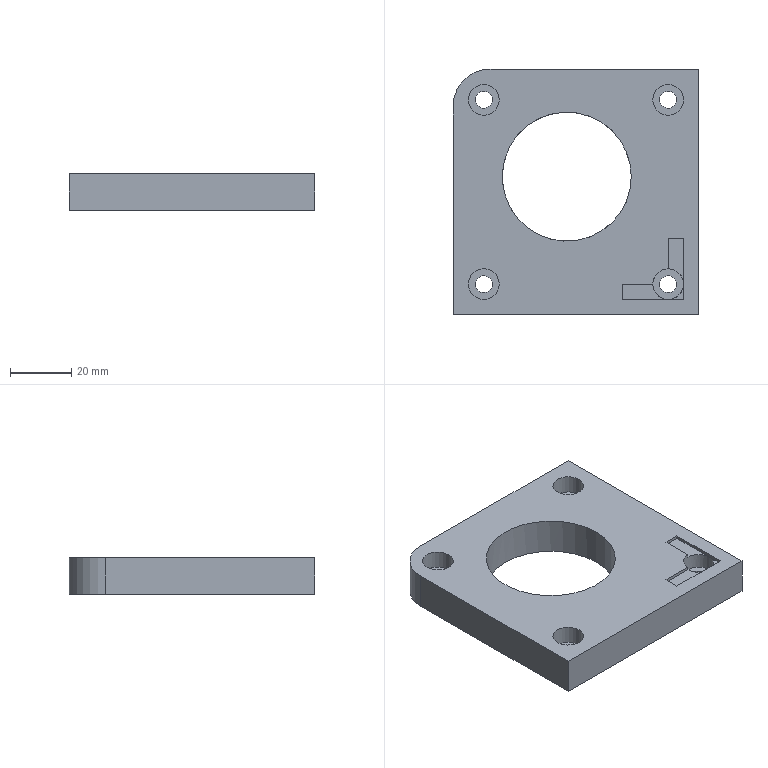Part | STEP file | solid 81 | 1 solid | 29 faces | box 80 x 80 x 12 mm | volume 57233 mm3 | plane 19 | cylinder 10 | commonest cylinder face diameters 5.5 x4 10 x4 24 x1 42 x1